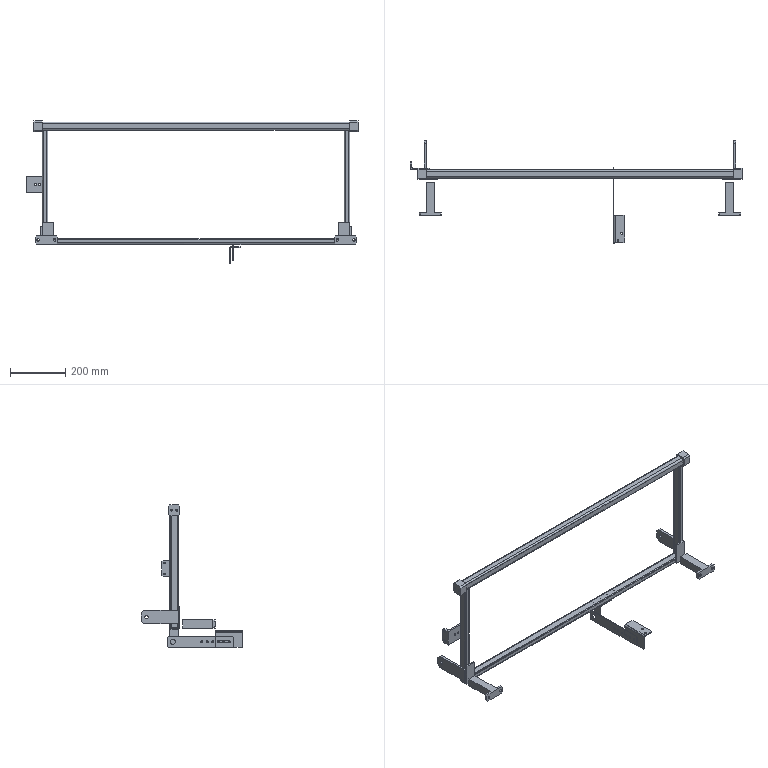Part | SolidWorks | 13 solids | 293 faces | box 1205 x 370 x 518 mm | volume 1223127 mm3 | plane 176 | cylinder 101 | cone 16 | commonest cylinder face diameters 4 x14 6.5 x14 8 x13 6.8 x12 7 x12 5 x8